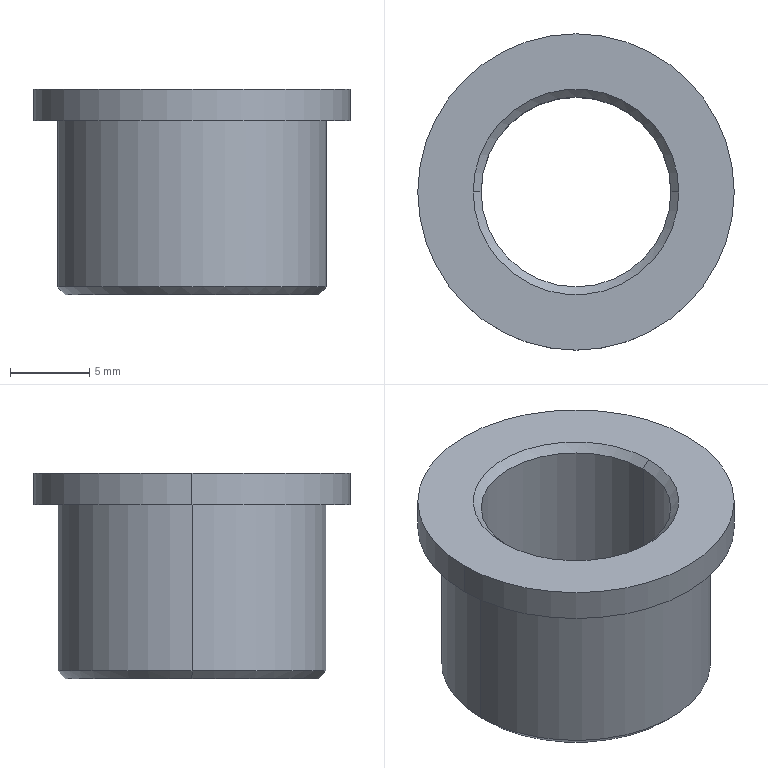Part | SolidWorks | features ICE 2, Chamfer 1, Extrusion 1 | 1 solid | 15 faces | box 20 x 20 x 13 mm | volume 1639 mm3 | cone 6 | cylinder 6 | plane 3 | commonest cylinder face diameters 12 x2 17 x2 20 x2
STEP:
#1=CARTESIAN_POINT('',(6.,0.,0.5));
#2=VERTEX_POINT('',#1);
#3=CARTESIAN_POINT('',(-6.,0.,0.5));
#4=VERTEX_POINT('',#3);
#5=CARTESIAN_POINT('',(0.,0.,0.5));
#6=DIRECTION('',(0.,0.,-1.));
#7=DIRECTION('',(1.,0.,0.));
#8=AXIS2_PLACEMENT_3D('',#5,#6,#7);
#9=CIRCLE('',#8,6.);
#10=EDGE_CURVE('',#2,#4,#9,.T.);
#11=ORIENTED_EDGE('',*,*,#10,.F.);
#12=CARTESIAN_POINT('',(6.5,0.,0.));
#13=VERTEX_POINT('',#12);
#14=CARTESIAN_POINT('',(6.,0.,0.5));
#15=DIRECTION('',(0.7071,0.,-0.7071));
#16=VECTOR('',#15,1000.);
#17=LINE('',#14,#16);
#18=EDGE_CURVE('',#2,#13,#17,.T.);
#19=ORIENTED_EDGE('',*,*,#18,.T.);
#20=CARTESIAN_POINT('',(-6.5,0.,0.));
#21=VERTEX_POINT('',#20);
#22=CARTESIAN_POINT('',(0.,0.,0.));
#23=DIRECTION('',(0.,0.,1.));
#24=DIRECTION('',(1.,0.,0.));
#25=AXIS2_PLACEMENT_3D('',#22,#23,#24);
#26=CIRCLE('',#25,6.5);
#27=EDGE_CURVE('',#21,#13,#26,.T.);
#28=ORIENTED_EDGE('',*,*,#27,.F.);
#29=CARTESIAN_POINT('',(-6.,0.,0.5));
#30=DIRECTION('',(-0.7071,0.,-0.7071));
#31=VECTOR('',#30,1000.);
#32=LINE('',#29,#31);
#33=EDGE_CURVE('',#4,#21,#32,.T.);
#34=ORIENTED_EDGE('',*,*,#33,.F.);
#35=EDGE_LOOP('',(#11,#19,#28,#34));
#36=FACE_OUTER_BOUND('',#35,.T.);
#37=CARTESIAN_POINT('',(0.,0.,0.5));
#38=DIRECTION('',(0.,0.,-1.));
#39=DIRECTION('',(-1.,0.,0.));
#40=AXIS2_PLACEMENT_3D('',#37,#38,#39);
#41=CONICAL_SURFACE('',#40,6.,0.7854);
#42=ADVANCED_FACE('',(#36),#41,.F.);
#43=CARTESIAN_POINT('',(-6.,0.,12.5));
#44=VERTEX_POINT('',#43);
#45=CARTESIAN_POINT('',(6.,0.,12.5));
#46=VERTEX_POINT('',#45);
#47=CARTESIAN_POINT('',(0.,0.,12.5));
#48=DIRECTION('',(0.,0.,1.));
#49=DIRECTION('',(1.,0.,0.));
#50=AXIS2_PLACEMENT_3D('',#47,#48,#49);
#51=CIRCLE('',#50,6.);
#52=EDGE_CURVE('',#44,#46,#51,.T.);
#53=ORIENTED_EDGE('',*,*,#52,.F.);
#54=CARTESIAN_POINT('',(-6.5,0.,13.));
#55=VERTEX_POINT('',#54);
#56=CARTESIAN_POINT('',(-6.,0.,12.5));
#57=DIRECTION('',(-0.7071,0.,0.7071));
#58=VECTOR('',#57,1000.);
#59=LINE('',#56,#58);
#60=EDGE_CURVE('',#44,#55,#59,.T.);
#61=ORIENTED_EDGE('',*,*,#60,.T.);
#62=CARTESIAN_POINT('',(6.5,0.,13.));
#63=VERTEX_POINT('',#62);
#64=CARTESIAN_POINT('',(0.,0.,13.));
#65=DIRECTION('',(0.,0.,-1.));
#66=DIRECTION('',(1.,0.,0.));
#67=AXIS2_PLACEMENT_3D('',#64,#65,#66);
#68=CIRCLE('',#67,6.5);
#69=EDGE_CURVE('',#63,#55,#68,.T.);
#70=ORIENTED_EDGE('',*,*,#69,.F.);
#71=CARTESIAN_POINT('',(6.,0.,12.5));
#72=DIRECTION('',(0.7071,0.,0.7071));
#73=VECTOR('',#72,1000.);
#74=LINE('',#71,#73);
#75=EDGE_CURVE('',#46,#63,#74,.T.);
#76=ORIENTED_EDGE('',*,*,#75,.F.);
#77=EDGE_LOOP('',(#53,#61,#70,#76));
#78=FACE_OUTER_BOUND('',#77,.T.);
#79=CARTESIAN_POINT('',(0.,0.,12.5));
#80=DIRECTION('',(0.,0.,1.));
#81=DIRECTION('',(1.,0.,0.));
#82=AXIS2_PLACEMENT_3D('',#79,#80,#81);
#83=CONICAL_SURFACE('',#82,6.,0.7854);
#84=ADVANCED_FACE('',(#78),#83,.F.);
#85=CARTESIAN_POINT('',(-8.,0.,0.));
#86=VERTEX_POINT('',#85);
#87=CARTESIAN_POINT('',(8.,0.,0.));
#88=VERTEX_POINT('',#87);
#89=CARTESIAN_POINT('',(0.,0.,0.));
#90=DIRECTION('',(0.,0.,-1.));
#91=DIRECTION('',(1.,0.,0.));
#92=AXIS2_PLACEMENT_3D('',#89,#90,#91);
#93=CIRCLE('',#92,8.);
#94=EDGE_CURVE('',#86,#88,#93,.T.);
#95=ORIENTED_EDGE('',*,*,#94,.F.);
#96=CARTESIAN_POINT('',(-8.5,0.,0.5));
#97=VERTEX_POINT('',#96);
#98=CARTESIAN_POINT('',(-8.5,0.,0.5));
#99=DIRECTION('',(-0.7071,0.,0.7071));
#100=VECTOR('',#99,1000.);
#101=LINE('',#98,#100);
#102=EDGE_CURVE('',#86,#97,#101,.T.);
#103=ORIENTED_EDGE('',*,*,#102,.T.);
#104=CARTESIAN_POINT('',(8.5,0.,0.5));
#105=VERTEX_POINT('',#104);
#106=CARTESIAN_POINT('',(0.,0.,0.5));
#107=DIRECTION('',(0.,0.,1.));
#108=DIRECTION('',(1.,0.,0.));
#109=AXIS2_PLACEMENT_3D('',#106,#107,#108);
#110=CIRCLE('',#109,8.5);
#111=EDGE_CURVE('',#105,#97,#110,.T.);
#112=ORIENTED_EDGE('',*,*,#111,.F.);
#113=CARTESIAN_POINT('',(8.5,0.,0.5));
#114=DIRECTION('',(0.7071,0.,0.7071));
#115=VECTOR('',#114,1000.);
#116=LINE('',#113,#115);
#117=EDGE_CURVE('',#88,#105,#116,.T.);
#118=ORIENTED_EDGE('',*,*,#117,.F.);
#119=EDGE_LOOP('',(#95,#103,#112,#118));
#120=FACE_OUTER_BOUND('',#119,.T.);
#121=CARTESIAN_POINT('',(0.,0.,0.5));
#122=DIRECTION('',(0.,0.,1.));
#123=DIRECTION('',(1.,0.,0.));
#124=AXIS2_PLACEMENT_3D('',#121,#122,#123);
#125=CONICAL_SURFACE('',#124,8.5,0.7854);
#126=ADVANCED_FACE('',(#120),#125,.T.);
#127=ORIENTED_EDGE('',*,*,#52,.T.);
#128=CARTESIAN_POINT('',(6.,0.,25.));
#129=DIRECTION('',(0.,0.,-1.));
#130=VECTOR('',#129,1000.);
#131=LINE('',#128,#130);
#132=EDGE_CURVE('',#46,#2,#131,.T.);
#133=ORIENTED_EDGE('',*,*,#132,.T.);
#134=ORIENTED_EDGE('',*,*,#10,.T.);
#135=CARTESIAN_POINT('',(-6.,0.,25.));
#136=DIRECTION('',(0.,0.,-1.));
#137=VECTOR('',#136,1000.);
#138=LINE('',#135,#137);
#139=EDGE_CURVE('',#44,#4,#138,.T.);
#140=ORIENTED_EDGE('',*,*,#139,.F.);
#141=EDGE_LOOP('',(#127,#133,#134,#140));
#142=FACE_OUTER_BOUND('',#141,.T.);
#143=CARTESIAN_POINT('',(0.,0.,25.));
#144=DIRECTION('',(0.,0.,-1.));
#145=DIRECTION('',(-1.,0.,0.));
#146=AXIS2_PLACEMENT_3D('',#143,#144,#145);
#147=CYLINDRICAL_SURFACE('',#146,6.);
#148=ADVANCED_FACE('',(#142),#147,.F.);
#149=CARTESIAN_POINT('',(10.,0.,11.));
#150=VERTEX_POINT('',#149);
#151=CARTESIAN_POINT('',(-10.,0.,11.));
#152=VERTEX_POINT('',#151);
#153=CARTESIAN_POINT('',(0.,0.,11.));
#154=DIRECTION('',(0.,0.,1.));
#155=DIRECTION('',(1.,0.,0.));
#156=AXIS2_PLACEMENT_3D('',#153,#154,#155);
#157=CIRCLE('',#156,10.);
#158=EDGE_CURVE('',#150,#152,#157,.T.);
#159=ORIENTED_EDGE('',*,*,#158,.T.);
#160=CARTESIAN_POINT('',(-10.,0.,13.));
#161=VERTEX_POINT('',#160);
#162=CARTESIAN_POINT('',(-10.,0.,11.));
#163=DIRECTION('',(0.,0.,1.));
#164=VECTOR('',#163,1000.);
#165=LINE('',#162,#164);
#166=EDGE_CURVE('',#152,#161,#165,.T.);
#167=ORIENTED_EDGE('',*,*,#166,.T.);
#168=CARTESIAN_POINT('',(10.,0.,13.));
#169=VERTEX_POINT('',#168);
#170=CARTESIAN_POINT('',(0.,0.,13.));
#171=DIRECTION('',(0.,0.,1.));
#172=DIRECTION('',(1.,0.,0.));
#173=AXIS2_PLACEMENT_3D('',#170,#171,#172);
#174=CIRCLE('',#173,10.);
#175=EDGE_CURVE('',#169,#161,#174,.T.);
#176=ORIENTED_EDGE('',*,*,#175,.F.);
#177=CARTESIAN_POINT('',(10.,0.,11.));
#178=DIRECTION('',(0.,0.,1.));
#179=VECTOR('',#178,1000.);
#180=LINE('',#177,#179);
#181=EDGE_CURVE('',#150,#169,#180,.T.);
#182=ORIENTED_EDGE('',*,*,#181,.F.);
#183=EDGE_LOOP('',(#159,#167,#176,#182));
#184=FACE_OUTER_BOUND('',#183,.T.);
#185=CARTESIAN_POINT('',(0.,0.,11.));
#186=DIRECTION('',(0.,0.,1.));
#187=DIRECTION('',(1.,0.,0.));
#188=AXIS2_PLACEMENT_3D('',#185,#186,#187);
#189=CYLINDRICAL_SURFACE('',#188,10.);
#190=ADVANCED_FACE('',(#184),#189,.T.);
#191=CARTESIAN_POINT('',(8.5,0.,11.));
#192=VERTEX_POINT('',#191);
#193=CARTESIAN_POINT('',(-8.5,0.,11.));
#194=VERTEX_POINT('',#193);
#195=CARTESIAN_POINT('',(0.,0.,11.));
#196=DIRECTION('',(0.,0.,1.));
#197=DIRECTION('',(1.,0.,0.));
#198=AXIS2_PLACEMENT_3D('',#195,#196,#197);
#199=CIRCLE('',#198,8.5);
#200=EDGE_CURVE('',#192,#194,#199,.T.);
#201=ORIENTED_EDGE('',*,*,#200,.F.);
#202=CARTESIAN_POINT('',(8.5,0.,13.));
#203=DIRECTION('',(0.,0.,-1.));
#204=VECTOR('',#203,1000.);
#205=LINE('',#202,#204);
#206=EDGE_CURVE('',#192,#105,#205,.T.);
#207=ORIENTED_EDGE('',*,*,#206,.T.);
#208=ORIENTED_EDGE('',*,*,#111,.T.);
#209=CARTESIAN_POINT('',(-8.5,0.,13.));
#210=DIRECTION('',(0.,0.,-1.));
#211=VECTOR('',#210,1000.);
#212=LINE('',#209,#211);
#213=EDGE_CURVE('',#194,#97,#212,.T.);
#214=ORIENTED_EDGE('',*,*,#213,.F.);
#215=EDGE_LOOP('',(#201,#207,#208,#214));
#216=FACE_OUTER_BOUND('',#215,.T.);
#217=CARTESIAN_POINT('',(0.,0.,13.));
#218=DIRECTION('',(0.,0.,-1.));
#219=DIRECTION('',(-1.,0.,0.));
#220=AXIS2_PLACEMENT_3D('',#217,#218,#219);
#221=CYLINDRICAL_SURFACE('',#220,8.5);
#222=ADVANCED_FACE('',(#216),#221,.T.);
#223=ORIENTED_EDGE('',*,*,#206,.F.);
#224=CARTESIAN_POINT('',(0.,0.,11.));
#225=DIRECTION('',(0.,0.,1.));
#226=DIRECTION('',(1.,0.,0.));
#227=AXIS2_PLACEMENT_3D('',#224,#225,#226);
#228=CIRCLE('',#227,8.5);
#229=EDGE_CURVE('',#194,#192,#228,.T.);
#230=ORIENTED_EDGE('',*,*,#229,.F.);
#231=ORIENTED_EDGE('',*,*,#213,.T.);
#232=CARTESIAN_POINT('',(0.,0.,0.5));
#233=DIRECTION('',(0.,0.,1.));
#234=DIRECTION('',(1.,0.,0.));
#235=AXIS2_PLACEMENT_3D('',#232,#233,#234);
#236=CIRCLE('',#235,8.5);
#237=EDGE_CURVE('',#97,#105,#236,.T.);
#238=ORIENTED_EDGE('',*,*,#237,.T.);
#239=EDGE_LOOP('',(#223,#230,#231,#238));
#240=FACE_OUTER_BOUND('',#239,.T.);
#241=CARTESIAN_POINT('',(0.,0.,13.));
#242=DIRECTION('',(0.,0.,-1.));
#243=DIRECTION('',(-1.,0.,0.));
#244=AXIS2_PLACEMENT_3D('',#241,#242,#243);
#245=CYLINDRICAL_SURFACE('',#244,8.5);
#246=ADVANCED_FACE('',(#240),#245,.T.);
#247=CARTESIAN_POINT('',(0.,0.,0.));
#248=DIRECTION('',(0.,0.,-1.));
#249=DIRECTION('',(1.,0.,0.));
#250=AXIS2_PLACEMENT_3D('',#247,#248,#249);
#251=CIRCLE('',#250,8.);
#252=EDGE_CURVE('',#88,#86,#251,.T.);
#253=ORIENTED_EDGE('',*,*,#252,.T.);
#254=ORIENTED_EDGE('',*,*,#94,.T.);
#255=EDGE_LOOP('',(#253,#254));
#256=FACE_OUTER_BOUND('',#255,.T.);
#257=ORIENTED_EDGE('',*,*,#27,.T.);
#258=CARTESIAN_POINT('',(0.,0.,0.));
#259=DIRECTION('',(0.,0.,1.));
#260=DIRECTION('',(1.,0.,0.));
#261=AXIS2_PLACEMENT_3D('',#258,#259,#260);
#262=CIRCLE('',#261,6.5);
#263=EDGE_CURVE('',#13,#21,#262,.T.);
#264=ORIENTED_EDGE('',*,*,#263,.T.);
#265=EDGE_LOOP('',(#257,#264));
#266=FACE_BOUND('',#265,.T.);
#267=CARTESIAN_POINT('',(0.,0.,0.));
#268=DIRECTION('',(0.,0.,1.));
#269=DIRECTION('',(1.,0.,0.));
#270=AXIS2_PLACEMENT_3D('',#267,#268,#269);
#271=PLANE('',#270);
#272=ADVANCED_FACE('',(#256,#266),#271,.F.);
#273=ORIENTED_EDGE('',*,*,#166,.F.);
#274=CARTESIAN_POINT('',(0.,0.,11.));
#275=DIRECTION('',(0.,0.,1.));
#276=DIRECTION('',(1.,0.,0.));
#277=AXIS2_PLACEMENT_3D('',#274,#275,#276);
#278=CIRCLE('',#277,10.);
#279=EDGE_CURVE('',#152,#150,#278,.T.);
#280=ORIENTED_EDGE('',*,*,#279,.T.);
#281=ORIENTED_EDGE('',*,*,#181,.T.);
#282=CARTESIAN_POINT('',(0.,0.,13.));
#283=DIRECTION('',(0.,0.,1.));
#284=DIRECTION('',(1.,0.,0.));
#285=AXIS2_PLACEMENT_3D('',#282,#283,#284);
#286=CIRCLE('',#285,10.);
#287=EDGE_CURVE('',#161,#169,#286,.T.);
#288=ORIENTED_EDGE('',*,*,#287,.F.);
#289=EDGE_LOOP('',(#273,#280,#281,#288));
#290=FACE_OUTER_BOUND('',#289,.T.);
#291=CARTESIAN_POINT('',(0.,0.,11.));
#292=DIRECTION('',(0.,0.,1.));
#293=DIRECTION('',(1.,0.,0.));
#294=AXIS2_PLACEMENT_3D('',#291,#292,#293);
#295=CYLINDRICAL_SURFACE('',#294,10.);
#296=ADVANCED_FACE('',(#290),#295,.T.);
#297=ORIENTED_EDGE('',*,*,#229,.T.);
#298=ORIENTED_EDGE('',*,*,#200,.T.);
#299=EDGE_LOOP('',(#297,#298));
#300=FACE_BOUND('',#299,.T.);
#301=ORIENTED_EDGE('',*,*,#158,.F.);
#302=ORIENTED_EDGE('',*,*,#279,.F.);
#303=EDGE_LOOP('',(#301,#302));
#304=FACE_OUTER_BOUND('',#303,.T.);
#305=CARTESIAN_POINT('',(0.,0.,11.));
#306=DIRECTION('',(0.,0.,1.));
#307=DIRECTION('',(1.,0.,0.));
#308=AXIS2_PLACEMENT_3D('',#305,#306,#307);
#309=PLANE('',#308);
#310=ADVANCED_FACE('',(#300,#304),#309,.F.);
#311=ORIENTED_EDGE('',*,*,#69,.T.);
#312=CARTESIAN_POINT('',(0.,0.,13.));
#313=DIRECTION('',(0.,0.,-1.));
#314=DIRECTION('',(1.,0.,0.));
#315=AXIS2_PLACEMENT_3D('',#312,#313,#314);
#316=CIRCLE('',#315,6.5);
#317=EDGE_CURVE('',#55,#63,#316,.T.);
#318=ORIENTED_EDGE('',*,*,#317,.T.);
#319=EDGE_LOOP('',(#311,#318));
#320=FACE_BOUND('',#319,.T.);
#321=ORIENTED_EDGE('',*,*,#175,.T.);
#322=ORIENTED_EDGE('',*,*,#287,.T.);
#323=EDGE_LOOP('',(#321,#322));
#324=FACE_OUTER_BOUND('',#323,.T.);
#325=CARTESIAN_POINT('',(0.,0.,13.));
#326=DIRECTION('',(0.,0.,1.));
#327=DIRECTION('',(1.,0.,0.));
#328=AXIS2_PLACEMENT_3D('',#325,#326,#327);
#329=PLANE('',#328);
#330=ADVANCED_FACE('',(#320,#324),#329,.T.);
#331=ORIENTED_EDGE('',*,*,#132,.F.);
#332=CARTESIAN_POINT('',(0.,0.,12.5));
#333=DIRECTION('',(0.,0.,1.));
#334=DIRECTION('',(1.,0.,0.));
#335=AXIS2_PLACEMENT_3D('',#332,#333,#334);
#336=CIRCLE('',#335,6.);
#337=EDGE_CURVE('',#46,#44,#336,.T.);
#338=ORIENTED_EDGE('',*,*,#337,.T.);
#339=ORIENTED_EDGE('',*,*,#139,.T.);
#340=CARTESIAN_POINT('',(0.,0.,0.5));
#341=DIRECTION('',(0.,0.,-1.));
#342=DIRECTION('',(1.,0.,0.));
#343=AXIS2_PLACEMENT_3D('',#340,#341,#342);
#344=CIRCLE('',#343,6.);
#345=EDGE_CURVE('',#4,#2,#344,.T.);
#346=ORIENTED_EDGE('',*,*,#345,.T.);
#347=EDGE_LOOP('',(#331,#338,#339,#346));
#348=FACE_OUTER_BOUND('',#347,.T.);
#349=CARTESIAN_POINT('',(0.,0.,25.));
#350=DIRECTION('',(0.,0.,-1.));
#351=DIRECTION('',(-1.,0.,0.));
#352=AXIS2_PLACEMENT_3D('',#349,#350,#351);
#353=CYLINDRICAL_SURFACE('',#352,6.);
#354=ADVANCED_FACE('',(#348),#353,.F.);
#355=ORIENTED_EDGE('',*,*,#102,.F.);
#356=ORIENTED_EDGE('',*,*,#252,.F.);
#357=ORIENTED_EDGE('',*,*,#117,.T.);
#358=ORIENTED_EDGE('',*,*,#237,.F.);
#359=EDGE_LOOP('',(#355,#356,#357,#358));
#360=FACE_OUTER_BOUND('',#359,.T.);
#361=CARTESIAN_POINT('',(0.,0.,0.5));
#362=DIRECTION('',(0.,0.,1.));
#363=DIRECTION('',(1.,0.,0.));
#364=AXIS2_PLACEMENT_3D('',#361,#362,#363);
#365=CONICAL_SURFACE('',#364,8.5,0.7854);
#366=ADVANCED_FACE('',(#360),#365,.T.);
#367=ORIENTED_EDGE('',*,*,#60,.F.);
#368=ORIENTED_EDGE('',*,*,#337,.F.);
#369=ORIENTED_EDGE('',*,*,#75,.T.);
#370=ORIENTED_EDGE('',*,*,#317,.F.);
#371=EDGE_LOOP('',(#367,#368,#369,#370));
#372=FACE_OUTER_BOUND('',#371,.T.);
#373=CARTESIAN_POINT('',(0.,0.,12.5));
#374=DIRECTION('',(0.,0.,1.));
#375=DIRECTION('',(1.,0.,0.));
#376=AXIS2_PLACEMENT_3D('',#373,#374,#375);
#377=CONICAL_SURFACE('',#376,6.,0.7854);
#378=ADVANCED_FACE('',(#372),#377,.F.);
#379=ORIENTED_EDGE('',*,*,#18,.F.);
#380=ORIENTED_EDGE('',*,*,#345,.F.);
#381=ORIENTED_EDGE('',*,*,#33,.T.);
#382=ORIENTED_EDGE('',*,*,#263,.F.);
#383=EDGE_LOOP('',(#379,#380,#381,#382));
#384=FACE_OUTER_BOUND('',#383,.T.);
#385=CARTESIAN_POINT('',(0.,0.,0.5));
#386=DIRECTION('',(0.,0.,-1.));
#387=DIRECTION('',(-1.,0.,0.));
#388=AXIS2_PLACEMENT_3D('',#385,#386,#387);
#389=CONICAL_SURFACE('',#388,6.,0.7854);
#390=ADVANCED_FACE('',(#384),#389,.F.);
#391=CLOSED_SHELL('',(#42,#84,#126,#148,#190,#222,#246,#272,#296,#310,#330,#354,#366,#378,#390));
#392=MANIFOLD_SOLID_BREP('',#391);
#393=CARTESIAN_POINT('',(0.,0.,0.));
#394=DIRECTION('',(0.,0.,1.));
#395=DIRECTION('',(1.,0.,0.));
#396=AXIS2_PLACEMENT_3D('',#393,#394,#395);
#397=(LENGTH_UNIT()NAMED_UNIT(*)SI_UNIT(.MILLI.,.METRE.));
#398=UNCERTAINTY_MEASURE_WITH_UNIT(LENGTH_MEASURE(0.00001),#397,'','');
#399=(NAMED_UNIT(*)PLANE_ANGLE_UNIT()SI_UNIT($,.RADIAN.));
#400=(NAMED_UNIT(*)SI_UNIT($,.STERADIAN.)SOLID_ANGLE_UNIT());
#401=(GEOMETRIC_REPRESENTATION_CONTEXT(3)GLOBAL_UNCERTAINTY_ASSIGNED_CONTEXT((#398))GLOBAL_UNIT_ASSIGNED_CONTEXT((#397,#399,#400))REPRESENTATION_CONTEXT('',''));
#402=ADVANCED_BREP_SHAPE_REPRESENTATION('',(#392,#396),#401);